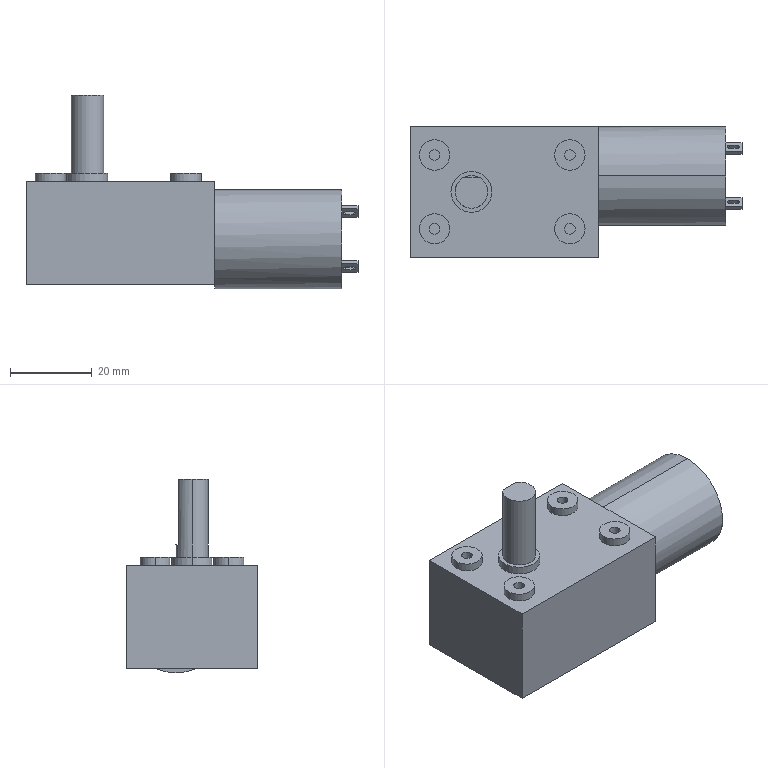Part | SolidWorks | features ICE 7, Extrusion 1 | 1 solid | 61 faces | box 81 x 32 x 47.2 mm | volume 52588 mm3 | plane 35 | cylinder 26 | commonest cylinder face diameters 2.6 x8 7.4 x8 1.039 x4 8 x2 10 x2 24.2 x2